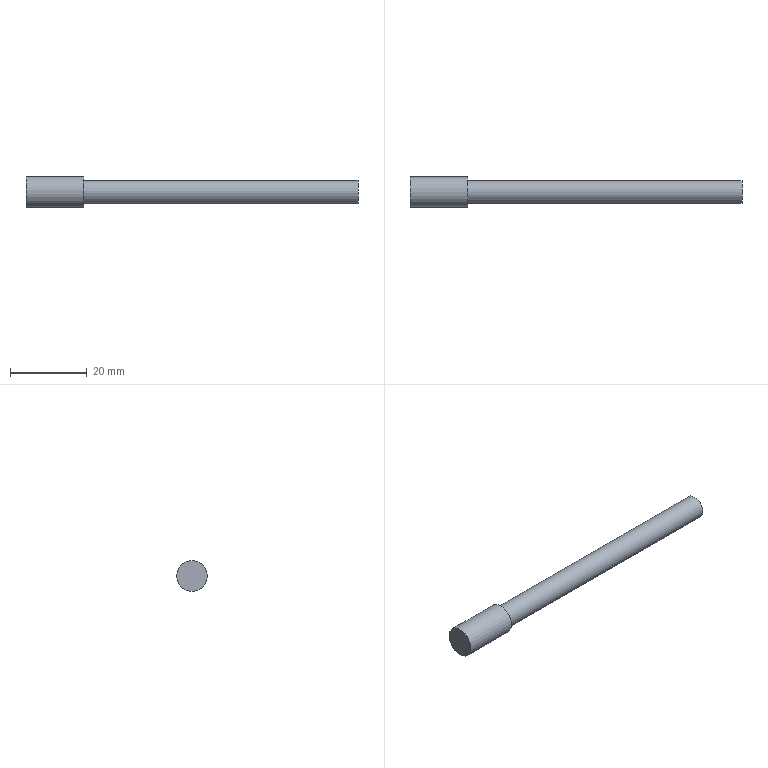Part | NX | features solid 2 | 1 solid | 5 faces | box 86.5 x 8 x 8 mm | volume 2776 mm3 | plane 3 | cylinder 2 | commonest cylinder face diameters 6 x1 8 x1
STEP:
#1=CARTESIAN_POINT('',(-95.,72.,28.));
#2=VERTEX_POINT('',#1);
#3=CARTESIAN_POINT('',(-95.,72.,25.));
#4=DIRECTION('',(-1.,0.,0.));
#5=DIRECTION('',(0.,0.,1.));
#6=AXIS2_PLACEMENT_3D('',#3,#4,#5);
#7=CIRCLE('',#6,3.);
#8=EDGE_CURVE('',#2,#2,#7,.T.);
#9=ORIENTED_EDGE('',*,*,#8,.F.);
#10=EDGE_LOOP('',(#9));
#11=FACE_BOUND('',#10,.T.);
#12=CARTESIAN_POINT('',(-23.5,72.,28.));
#13=VERTEX_POINT('',#12);
#14=CARTESIAN_POINT('',(-23.5,72.,25.));
#15=DIRECTION('',(1.,0.,0.));
#16=DIRECTION('',(0.,0.,1.));
#17=AXIS2_PLACEMENT_3D('',#14,#15,#16);
#18=CIRCLE('',#17,3.);
#19=EDGE_CURVE('',#13,#13,#18,.F.);
#20=ORIENTED_EDGE('',*,*,#19,.T.);
#21=EDGE_LOOP('',(#20));
#22=FACE_BOUND('',#21,.T.);
#23=CARTESIAN_POINT('',(-125.,72.,25.));
#24=DIRECTION('',(1.,0.,0.));
#25=DIRECTION('',(0.,0.,1.));
#26=AXIS2_PLACEMENT_3D('',#23,#24,#25);
#27=CYLINDRICAL_SURFACE('',#26,3.);
#28=ADVANCED_FACE('',(#11,#22),#27,.T.);
#29=ORIENTED_EDGE('',*,*,#19,.F.);
#30=EDGE_LOOP('',(#29));
#31=FACE_BOUND('',#30,.T.);
#32=CARTESIAN_POINT('',(-23.5,3.,17.5));
#33=DIRECTION('',(1.,0.,0.));
#34=DIRECTION('',(0.,0.,1.));
#35=AXIS2_PLACEMENT_3D('',#32,#33,#34);
#36=PLANE('',#35);
#37=ADVANCED_FACE('',(#31),#36,.T.);
#38=CARTESIAN_POINT('',(-95.,72.,29.));
#39=VERTEX_POINT('',#38);
#40=CARTESIAN_POINT('',(-95.,72.,25.));
#41=DIRECTION('',(-1.,0.,0.));
#42=DIRECTION('',(0.,0.,1.));
#43=AXIS2_PLACEMENT_3D('',#40,#41,#42);
#44=CIRCLE('',#43,4.);
#45=EDGE_CURVE('',#39,#39,#44,.T.);
#46=ORIENTED_EDGE('',*,*,#45,.F.);
#47=EDGE_LOOP('',(#46));
#48=FACE_BOUND('',#47,.T.);
#49=ORIENTED_EDGE('',*,*,#8,.T.);
#50=EDGE_LOOP('',(#49));
#51=FACE_BOUND('',#50,.T.);
#52=CARTESIAN_POINT('',(-95.,72.,25.));
#53=DIRECTION('',(1.,0.,0.));
#54=DIRECTION('',(0.,0.,1.));
#55=AXIS2_PLACEMENT_3D('',#52,#53,#54);
#56=PLANE('',#55);
#57=ADVANCED_FACE('',(#48,#51),#56,.T.);
#58=ORIENTED_EDGE('',*,*,#45,.T.);
#59=EDGE_LOOP('',(#58));
#60=FACE_BOUND('',#59,.T.);
#61=CARTESIAN_POINT('',(-110.,72.,29.));
#62=VERTEX_POINT('',#61);
#63=CARTESIAN_POINT('',(-110.,72.,25.));
#64=DIRECTION('',(-1.,0.,0.));
#65=DIRECTION('',(0.,0.,1.));
#66=AXIS2_PLACEMENT_3D('',#63,#64,#65);
#67=CIRCLE('',#66,4.);
#68=EDGE_CURVE('',#62,#62,#67,.T.);
#69=ORIENTED_EDGE('',*,*,#68,.F.);
#70=EDGE_LOOP('',(#69));
#71=FACE_BOUND('',#70,.T.);
#72=CARTESIAN_POINT('',(-95.,72.,25.));
#73=DIRECTION('',(-1.,0.,0.));
#74=DIRECTION('',(0.,0.,-1.));
#75=AXIS2_PLACEMENT_3D('',#72,#73,#74);
#76=CYLINDRICAL_SURFACE('',#75,4.);
#77=ADVANCED_FACE('',(#60,#71),#76,.T.);
#78=ORIENTED_EDGE('',*,*,#68,.T.);
#79=EDGE_LOOP('',(#78));
#80=FACE_BOUND('',#79,.T.);
#81=CARTESIAN_POINT('',(-110.,72.,25.));
#82=DIRECTION('',(-1.,0.,0.));
#83=DIRECTION('',(0.,0.,-1.));
#84=AXIS2_PLACEMENT_3D('',#81,#82,#83);
#85=PLANE('',#84);
#86=ADVANCED_FACE('',(#80),#85,.T.);
#87=CLOSED_SHELL('',(#28,#37,#57,#77,#86));
#88=MANIFOLD_SOLID_BREP('',#87);
#89=(LENGTH_UNIT()NAMED_UNIT(*)SI_UNIT(.MILLI.,.METRE.));
#90=UNCERTAINTY_MEASURE_WITH_UNIT(LENGTH_MEASURE(0.00001),#89,'','');
#91=(NAMED_UNIT(*)PLANE_ANGLE_UNIT()SI_UNIT($,.RADIAN.));
#92=(NAMED_UNIT(*)SI_UNIT($,.STERADIAN.)SOLID_ANGLE_UNIT());
#93=(GEOMETRIC_REPRESENTATION_CONTEXT(3)GLOBAL_UNCERTAINTY_ASSIGNED_CONTEXT((#90))GLOBAL_UNIT_ASSIGNED_CONTEXT((#89,#91,#92))REPRESENTATION_CONTEXT('',''));
#94=ADVANCED_BREP_SHAPE_REPRESENTATION('',(#88),#93);